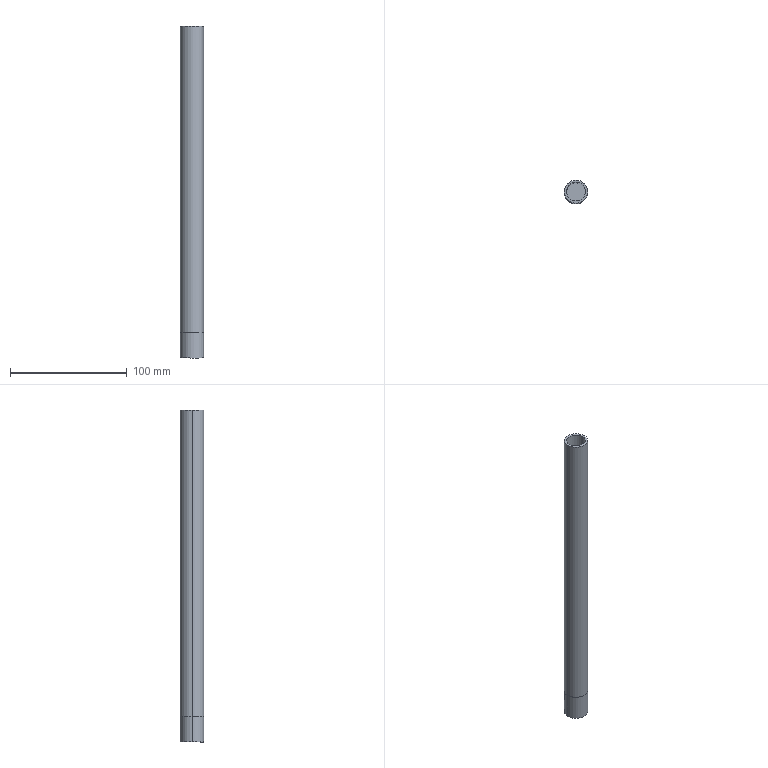Part | SolidWorks | features BaseBody 2 | 2 solids | 17 faces | box 20 x 20 x 284 mm | volume 37985 mm3 | cylinder 10 | plane 5 | cone 2 | commonest cylinder face diameters 16 x4 20 x4 5 x2
STEP:
#1=CARTESIAN_POINT('',(-12.135,0.8028,131.));
#2=VERTEX_POINT('',#1);
#3=CARTESIAN_POINT('',(3.865,0.8028,131.));
#4=VERTEX_POINT('',#3);
#5=CARTESIAN_POINT('',(-4.135,0.8028,131.));
#6=DIRECTION('',(0.,0.,1.));
#7=DIRECTION('',(1.,0.,0.));
#8=AXIS2_PLACEMENT_3D('',#5,#6,#7);
#9=CIRCLE('',#8,8.);
#10=EDGE_CURVE('',#2,#4,#9,.T.);
#11=ORIENTED_EDGE('',*,*,#10,.T.);
#12=CARTESIAN_POINT('',(3.865,0.8028,-131.));
#13=VERTEX_POINT('',#12);
#14=CARTESIAN_POINT('',(3.865,0.8028,131.));
#15=DIRECTION('',(0.,0.,-1.));
#16=VECTOR('',#15,1000.);
#17=LINE('',#14,#16);
#18=EDGE_CURVE('',#4,#13,#17,.T.);
#19=ORIENTED_EDGE('',*,*,#18,.T.);
#20=CARTESIAN_POINT('',(-12.135,0.8028,-131.));
#21=VERTEX_POINT('',#20);
#22=CARTESIAN_POINT('',(-4.135,0.8028,-131.));
#23=DIRECTION('',(0.,0.,1.));
#24=DIRECTION('',(1.,0.,0.));
#25=AXIS2_PLACEMENT_3D('',#22,#23,#24);
#26=CIRCLE('',#25,8.);
#27=EDGE_CURVE('',#21,#13,#26,.T.);
#28=ORIENTED_EDGE('',*,*,#27,.F.);
#29=CARTESIAN_POINT('',(-12.135,0.8028,131.));
#30=DIRECTION('',(0.,0.,-1.));
#31=VECTOR('',#30,1000.);
#32=LINE('',#29,#31);
#33=EDGE_CURVE('',#2,#21,#32,.T.);
#34=ORIENTED_EDGE('',*,*,#33,.F.);
#35=EDGE_LOOP('',(#11,#19,#28,#34));
#36=FACE_OUTER_BOUND('',#35,.T.);
#37=CARTESIAN_POINT('',(-4.135,0.8028,131.));
#38=DIRECTION('',(0.,0.,-1.));
#39=DIRECTION('',(-1.,0.,0.));
#40=AXIS2_PLACEMENT_3D('',#37,#38,#39);
#41=CYLINDRICAL_SURFACE('',#40,8.);
#42=ADVANCED_FACE('',(#36),#41,.F.);
#43=CARTESIAN_POINT('',(5.865,0.8028,131.));
#44=VERTEX_POINT('',#43);
#45=CARTESIAN_POINT('',(-14.135,0.8028,131.));
#46=VERTEX_POINT('',#45);
#47=CARTESIAN_POINT('',(-4.135,0.8028,131.));
#48=DIRECTION('',(0.,0.,1.));
#49=DIRECTION('',(1.,0.,0.));
#50=AXIS2_PLACEMENT_3D('',#47,#48,#49);
#51=CIRCLE('',#50,10.);
#52=EDGE_CURVE('',#44,#46,#51,.T.);
#53=ORIENTED_EDGE('',*,*,#52,.F.);
#54=CARTESIAN_POINT('',(5.865,0.8028,-131.));
#55=VERTEX_POINT('',#54);
#56=CARTESIAN_POINT('',(5.865,0.8028,131.));
#57=DIRECTION('',(0.,0.,-1.));
#58=VECTOR('',#57,1000.);
#59=LINE('',#56,#58);
#60=EDGE_CURVE('',#44,#55,#59,.T.);
#61=ORIENTED_EDGE('',*,*,#60,.T.);
#62=CARTESIAN_POINT('',(-14.135,0.8028,-131.));
#63=VERTEX_POINT('',#62);
#64=CARTESIAN_POINT('',(-4.135,0.8028,-131.));
#65=DIRECTION('',(0.,0.,1.));
#66=DIRECTION('',(1.,0.,0.));
#67=AXIS2_PLACEMENT_3D('',#64,#65,#66);
#68=CIRCLE('',#67,10.);
#69=EDGE_CURVE('',#55,#63,#68,.T.);
#70=ORIENTED_EDGE('',*,*,#69,.T.);
#71=CARTESIAN_POINT('',(-14.135,0.8028,131.));
#72=DIRECTION('',(0.,0.,-1.));
#73=VECTOR('',#72,1000.);
#74=LINE('',#71,#73);
#75=EDGE_CURVE('',#46,#63,#74,.T.);
#76=ORIENTED_EDGE('',*,*,#75,.F.);
#77=EDGE_LOOP('',(#53,#61,#70,#76));
#78=FACE_OUTER_BOUND('',#77,.T.);
#79=CARTESIAN_POINT('',(-4.135,0.8028,131.));
#80=DIRECTION('',(0.,0.,-1.));
#81=DIRECTION('',(-1.,0.,0.));
#82=AXIS2_PLACEMENT_3D('',#79,#80,#81);
#83=CYLINDRICAL_SURFACE('',#82,10.);
#84=ADVANCED_FACE('',(#78),#83,.T.);
#85=CARTESIAN_POINT('',(-4.135,0.8028,131.));
#86=DIRECTION('',(0.,0.,1.));
#87=DIRECTION('',(1.,0.,0.));
#88=AXIS2_PLACEMENT_3D('',#85,#86,#87);
#89=CIRCLE('',#88,10.);
#90=EDGE_CURVE('',#46,#44,#89,.T.);
#91=ORIENTED_EDGE('',*,*,#90,.T.);
#92=ORIENTED_EDGE('',*,*,#52,.T.);
#93=EDGE_LOOP('',(#91,#92));
#94=FACE_OUTER_BOUND('',#93,.T.);
#95=ORIENTED_EDGE('',*,*,#10,.F.);
#96=CARTESIAN_POINT('',(-4.135,0.8028,131.));
#97=DIRECTION('',(0.,0.,1.));
#98=DIRECTION('',(1.,0.,0.));
#99=AXIS2_PLACEMENT_3D('',#96,#97,#98);
#100=CIRCLE('',#99,8.);
#101=EDGE_CURVE('',#4,#2,#100,.T.);
#102=ORIENTED_EDGE('',*,*,#101,.F.);
#103=EDGE_LOOP('',(#95,#102));
#104=FACE_BOUND('',#103,.T.);
#105=CARTESIAN_POINT('',(-4.135,0.8028,131.));
#106=DIRECTION('',(0.,0.,1.));
#107=DIRECTION('',(1.,0.,0.));
#108=AXIS2_PLACEMENT_3D('',#105,#106,#107);
#109=PLANE('',#108);
#110=ADVANCED_FACE('',(#94,#104),#109,.T.);
#111=CARTESIAN_POINT('',(-4.135,0.8028,-131.));
#112=DIRECTION('',(0.,0.,1.));
#113=DIRECTION('',(1.,0.,0.));
#114=AXIS2_PLACEMENT_3D('',#111,#112,#113);
#115=CIRCLE('',#114,10.);
#116=EDGE_CURVE('',#63,#55,#115,.T.);
#117=ORIENTED_EDGE('',*,*,#116,.F.);
#118=ORIENTED_EDGE('',*,*,#69,.F.);
#119=EDGE_LOOP('',(#117,#118));
#120=FACE_OUTER_BOUND('',#119,.T.);
#121=ORIENTED_EDGE('',*,*,#27,.T.);
#122=CARTESIAN_POINT('',(-4.135,0.8028,-131.));
#123=DIRECTION('',(0.,0.,1.));
#124=DIRECTION('',(1.,0.,0.));
#125=AXIS2_PLACEMENT_3D('',#122,#123,#124);
#126=CIRCLE('',#125,8.);
#127=EDGE_CURVE('',#13,#21,#126,.T.);
#128=ORIENTED_EDGE('',*,*,#127,.T.);
#129=EDGE_LOOP('',(#121,#128));
#130=FACE_BOUND('',#129,.T.);
#131=CARTESIAN_POINT('',(-4.135,0.8028,-131.));
#132=DIRECTION('',(0.,0.,1.));
#133=DIRECTION('',(1.,0.,0.));
#134=AXIS2_PLACEMENT_3D('',#131,#132,#133);
#135=PLANE('',#134);
#136=ADVANCED_FACE('',(#120,#130),#135,.F.);
#137=ORIENTED_EDGE('',*,*,#60,.F.);
#138=ORIENTED_EDGE('',*,*,#90,.F.);
#139=ORIENTED_EDGE('',*,*,#75,.T.);
#140=ORIENTED_EDGE('',*,*,#116,.T.);
#141=EDGE_LOOP('',(#137,#138,#139,#140));
#142=FACE_OUTER_BOUND('',#141,.T.);
#143=CARTESIAN_POINT('',(-4.135,0.8028,131.));
#144=DIRECTION('',(0.,0.,-1.));
#145=DIRECTION('',(-1.,0.,0.));
#146=AXIS2_PLACEMENT_3D('',#143,#144,#145);
#147=CYLINDRICAL_SURFACE('',#146,10.);
#148=ADVANCED_FACE('',(#142),#147,.T.);
#149=ORIENTED_EDGE('',*,*,#18,.F.);
#150=ORIENTED_EDGE('',*,*,#101,.T.);
#151=ORIENTED_EDGE('',*,*,#33,.T.);
#152=ORIENTED_EDGE('',*,*,#127,.F.);
#153=EDGE_LOOP('',(#149,#150,#151,#152));
#154=FACE_OUTER_BOUND('',#153,.T.);
#155=CARTESIAN_POINT('',(-4.135,0.8028,131.));
#156=DIRECTION('',(0.,0.,-1.));
#157=DIRECTION('',(-1.,0.,0.));
#158=AXIS2_PLACEMENT_3D('',#155,#156,#157);
#159=CYLINDRICAL_SURFACE('',#158,8.);
#160=ADVANCED_FACE('',(#154),#159,.F.);
#161=CLOSED_SHELL('',(#42,#84,#110,#136,#148,#160));
#162=MANIFOLD_SOLID_BREP('',#161);
#163=CARTESIAN_POINT('',(-1.636,0.8812,-145.));
#164=VERTEX_POINT('',#163);
#165=CARTESIAN_POINT('',(-6.634,0.7244,-145.));
#166=VERTEX_POINT('',#165);
#167=CARTESIAN_POINT('',(-4.135,0.8028,-145.));
#168=DIRECTION('',(0.,0.,-1.));
#169=DIRECTION('',(-0.9995,-0.03135,0.));
#170=AXIS2_PLACEMENT_3D('',#167,#168,#169);
#171=CIRCLE('',#170,2.5);
#172=EDGE_CURVE('',#164,#166,#171,.T.);
#173=ORIENTED_EDGE('',*,*,#172,.F.);
#174=CARTESIAN_POINT('',(-1.636,0.8812,-153.));
#175=VERTEX_POINT('',#174);
#176=CARTESIAN_POINT('',(-1.636,0.8812,-153.));
#177=DIRECTION('',(0.,0.,-1.));
#178=VECTOR('',#177,1000.);
#179=LINE('',#176,#178);
#180=EDGE_CURVE('',#164,#175,#179,.T.);
#181=ORIENTED_EDGE('',*,*,#180,.T.);
#182=CARTESIAN_POINT('',(-6.634,0.7244,-153.));
#183=VERTEX_POINT('',#182);
#184=CARTESIAN_POINT('',(-4.135,0.8028,-153.));
#185=DIRECTION('',(0.,0.,-1.));
#186=DIRECTION('',(-0.9995,-0.03135,0.));
#187=AXIS2_PLACEMENT_3D('',#184,#185,#186);
#188=CIRCLE('',#187,2.5);
#189=EDGE_CURVE('',#175,#183,#188,.T.);
#190=ORIENTED_EDGE('',*,*,#189,.T.);
#191=CARTESIAN_POINT('',(-6.634,0.7244,-153.));
#192=DIRECTION('',(0.,0.,-1.));
#193=VECTOR('',#192,1000.);
#194=LINE('',#191,#193);
#195=EDGE_CURVE('',#166,#183,#194,.T.);
#196=ORIENTED_EDGE('',*,*,#195,.F.);
#197=EDGE_LOOP('',(#173,#181,#190,#196));
#198=FACE_OUTER_BOUND('',#197,.T.);
#199=CARTESIAN_POINT('',(-4.135,0.8028,-153.));
#200=DIRECTION('',(0.,0.,-1.));
#201=DIRECTION('',(-0.9995,-0.03135,0.));
#202=AXIS2_PLACEMENT_3D('',#199,#200,#201);
#203=CYLINDRICAL_SURFACE('',#202,2.5);
#204=ADVANCED_FACE('',(#198),#203,.F.);
#205=CARTESIAN_POINT('',(-4.135,0.8028,-143.498));
#206=VERTEX_POINT('',#205);
#207=CARTESIAN_POINT('',(-6.634,0.7244,-145.));
#208=DIRECTION('',(-0.8567,-0.02688,-0.515));
#209=VECTOR('',#208,1000.);
#210=LINE('',#207,#209);
#211=EDGE_CURVE('',#206,#166,#210,.T.);
#212=ORIENTED_EDGE('',*,*,#211,.F.);
#213=CARTESIAN_POINT('',(-1.636,0.8812,-145.));
#214=DIRECTION('',(0.8567,0.02688,-0.515));
#215=VECTOR('',#214,1000.);
#216=LINE('',#213,#215);
#217=EDGE_CURVE('',#206,#164,#216,.T.);
#218=ORIENTED_EDGE('',*,*,#217,.T.);
#219=ORIENTED_EDGE('',*,*,#172,.T.);
#220=EDGE_LOOP('',(#212,#218,#219));
#221=FACE_OUTER_BOUND('',#220,.T.);
#222=CARTESIAN_POINT('',(-4.135,0.8028,-145.));
#223=DIRECTION('',(0.,0.,-1.));
#224=DIRECTION('',(-0.9995,-0.03135,0.));
#225=AXIS2_PLACEMENT_3D('',#222,#223,#224);
#226=CONICAL_SURFACE('',#225,2.5,1.03);
#227=ADVANCED_FACE('',(#221),#226,.F.);
#228=CARTESIAN_POINT('',(5.86,1.116,-153.));
#229=VERTEX_POINT('',#228);
#230=CARTESIAN_POINT('',(-14.13,0.4893,-153.));
#231=VERTEX_POINT('',#230);
#232=CARTESIAN_POINT('',(-4.135,0.8028,-153.));
#233=DIRECTION('',(0.,0.,1.));
#234=DIRECTION('',(0.9995,0.03135,0.));
#235=AXIS2_PLACEMENT_3D('',#232,#233,#234);
#236=CIRCLE('',#235,10.);
#237=EDGE_CURVE('',#229,#231,#236,.T.);
#238=ORIENTED_EDGE('',*,*,#237,.T.);
#239=CARTESIAN_POINT('',(-14.13,0.4893,-131.));
#240=VERTEX_POINT('',#239);
#241=CARTESIAN_POINT('',(-14.13,0.4893,-153.));
#242=DIRECTION('',(0.,0.,1.));
#243=VECTOR('',#242,1000.);
#244=LINE('',#241,#243);
#245=EDGE_CURVE('',#231,#240,#244,.T.);
#246=ORIENTED_EDGE('',*,*,#245,.T.);
#247=CARTESIAN_POINT('',(5.86,1.116,-131.));
#248=VERTEX_POINT('',#247);
#249=CARTESIAN_POINT('',(-4.135,0.8028,-131.));
#250=DIRECTION('',(0.,0.,1.));
#251=DIRECTION('',(0.9995,0.03135,0.));
#252=AXIS2_PLACEMENT_3D('',#249,#250,#251);
#253=CIRCLE('',#252,10.);
#254=EDGE_CURVE('',#248,#240,#253,.T.);
#255=ORIENTED_EDGE('',*,*,#254,.F.);
#256=CARTESIAN_POINT('',(5.86,1.116,-153.));
#257=DIRECTION('',(0.,0.,1.));
#258=VECTOR('',#257,1000.);
#259=LINE('',#256,#258);
#260=EDGE_CURVE('',#229,#248,#259,.T.);
#261=ORIENTED_EDGE('',*,*,#260,.F.);
#262=EDGE_LOOP('',(#238,#246,#255,#261));
#263=FACE_OUTER_BOUND('',#262,.T.);
#264=CARTESIAN_POINT('',(-4.135,0.8028,-153.));
#265=DIRECTION('',(0.,0.,1.));
#266=DIRECTION('',(0.9995,0.03135,0.));
#267=AXIS2_PLACEMENT_3D('',#264,#265,#266);
#268=CYLINDRICAL_SURFACE('',#267,10.);
#269=ADVANCED_FACE('',(#263),#268,.T.);
#270=CARTESIAN_POINT('',(3.861,1.054,-123.));
#271=VERTEX_POINT('',#270);
#272=CARTESIAN_POINT('',(-12.131,0.552,-123.));
#273=VERTEX_POINT('',#272);
#274=CARTESIAN_POINT('',(-4.135,0.8028,-123.));
#275=DIRECTION('',(0.,0.,1.));
#276=DIRECTION('',(0.9995,0.03135,0.));
#277=AXIS2_PLACEMENT_3D('',#274,#275,#276);
#278=CIRCLE('',#277,8.);
#279=EDGE_CURVE('',#271,#273,#278,.T.);
#280=ORIENTED_EDGE('',*,*,#279,.F.);
#281=CARTESIAN_POINT('',(3.861,1.054,-131.));
#282=VERTEX_POINT('',#281);
#283=CARTESIAN_POINT('',(3.861,1.054,-123.));
#284=DIRECTION('',(0.,0.,-1.));
#285=VECTOR('',#284,1000.);
#286=LINE('',#283,#285);
#287=EDGE_CURVE('',#271,#282,#286,.T.);
#288=ORIENTED_EDGE('',*,*,#287,.T.);
#289=CARTESIAN_POINT('',(-12.131,0.552,-131.));
#290=VERTEX_POINT('',#289);
#291=CARTESIAN_POINT('',(-4.135,0.8028,-131.));
#292=DIRECTION('',(0.,0.,1.));
#293=DIRECTION('',(0.9995,0.03135,0.));
#294=AXIS2_PLACEMENT_3D('',#291,#292,#293);
#295=CIRCLE('',#294,8.);
#296=EDGE_CURVE('',#282,#290,#295,.T.);
#297=ORIENTED_EDGE('',*,*,#296,.T.);
#298=CARTESIAN_POINT('',(-12.131,0.552,-123.));
#299=DIRECTION('',(0.,0.,-1.));
#300=VECTOR('',#299,1000.);
#301=LINE('',#298,#300);
#302=EDGE_CURVE('',#273,#290,#301,.T.);
#303=ORIENTED_EDGE('',*,*,#302,.F.);
#304=EDGE_LOOP('',(#280,#288,#297,#303));
#305=FACE_OUTER_BOUND('',#304,.T.);
#306=CARTESIAN_POINT('',(-4.135,0.8028,-123.));
#307=DIRECTION('',(0.,0.,-1.));
#308=DIRECTION('',(-0.9995,-0.03135,0.));
#309=AXIS2_PLACEMENT_3D('',#306,#307,#308);
#310=CYLINDRICAL_SURFACE('',#309,8.);
#311=ADVANCED_FACE('',(#305),#310,.T.);
#312=ORIENTED_EDGE('',*,*,#287,.F.);
#313=CARTESIAN_POINT('',(-4.135,0.8028,-123.));
#314=DIRECTION('',(0.,0.,1.));
#315=DIRECTION('',(0.9995,0.03135,0.));
#316=AXIS2_PLACEMENT_3D('',#313,#314,#315);
#317=CIRCLE('',#316,8.);
#318=EDGE_CURVE('',#273,#271,#317,.T.);
#319=ORIENTED_EDGE('',*,*,#318,.F.);
#320=ORIENTED_EDGE('',*,*,#302,.T.);
#321=CARTESIAN_POINT('',(-4.135,0.8028,-131.));
#322=DIRECTION('',(0.,0.,1.));
#323=DIRECTION('',(0.9995,0.03135,0.));
#324=AXIS2_PLACEMENT_3D('',#321,#322,#323);
#325=CIRCLE('',#324,8.);
#326=EDGE_CURVE('',#290,#282,#325,.T.);
#327=ORIENTED_EDGE('',*,*,#326,.T.);
#328=EDGE_LOOP('',(#312,#319,#320,#327));
#329=FACE_OUTER_BOUND('',#328,.T.);
#330=CARTESIAN_POINT('',(-4.135,0.8028,-123.));
#331=DIRECTION('',(0.,0.,-1.));
#332=DIRECTION('',(-0.9995,-0.03135,0.));
#333=AXIS2_PLACEMENT_3D('',#330,#331,#332);
#334=CYLINDRICAL_SURFACE('',#333,8.);
#335=ADVANCED_FACE('',(#329),#334,.T.);
#336=ORIENTED_EDGE('',*,*,#318,.T.);
#337=ORIENTED_EDGE('',*,*,#279,.T.);
#338=EDGE_LOOP('',(#336,#337));
#339=FACE_OUTER_BOUND('',#338,.T.);
#340=CARTESIAN_POINT('',(-4.135,0.8028,-123.));
#341=DIRECTION('',(0.,0.,1.));
#342=DIRECTION('',(0.9995,0.03135,0.));
#343=AXIS2_PLACEMENT_3D('',#340,#341,#342);
#344=PLANE('',#343);
#345=ADVANCED_FACE('',(#339),#344,.T.);
#346=ORIENTED_EDGE('',*,*,#245,.F.);
#347=CARTESIAN_POINT('',(-4.135,0.8028,-153.));
#348=DIRECTION('',(0.,0.,1.));
#349=DIRECTION('',(0.9995,0.03135,0.));
#350=AXIS2_PLACEMENT_3D('',#347,#348,#349);
#351=CIRCLE('',#350,10.);
#352=EDGE_CURVE('',#231,#229,#351,.T.);
#353=ORIENTED_EDGE('',*,*,#352,.T.);
#354=ORIENTED_EDGE('',*,*,#260,.T.);
#355=CARTESIAN_POINT('',(-4.135,0.8028,-131.));
#356=DIRECTION('',(0.,0.,1.));
#357=DIRECTION('',(0.9995,0.03135,0.));
#358=AXIS2_PLACEMENT_3D('',#355,#356,#357);
#359=CIRCLE('',#358,10.);
#360=EDGE_CURVE('',#240,#248,#359,.T.);
#361=ORIENTED_EDGE('',*,*,#360,.F.);
#362=EDGE_LOOP('',(#346,#353,#354,#361));
#363=FACE_OUTER_BOUND('',#362,.T.);
#364=CARTESIAN_POINT('',(-4.135,0.8028,-153.));
#365=DIRECTION('',(0.,0.,1.));
#366=DIRECTION('',(0.9995,0.03135,0.));
#367=AXIS2_PLACEMENT_3D('',#364,#365,#366);
#368=CYLINDRICAL_SURFACE('',#367,10.);
#369=ADVANCED_FACE('',(#363),#368,.T.);
#370=CARTESIAN_POINT('',(-4.135,0.8028,-153.));
#371=DIRECTION('',(0.,0.,-1.));
#372=DIRECTION('',(-0.9995,-0.03135,0.));
#373=AXIS2_PLACEMENT_3D('',#370,#371,#372);
#374=CIRCLE('',#373,2.5);
#375=EDGE_CURVE('',#183,#175,#374,.T.);
#376=ORIENTED_EDGE('',*,*,#375,.F.);
#377=ORIENTED_EDGE('',*,*,#189,.F.);
#378=EDGE_LOOP('',(#376,#377));
#379=FACE_BOUND('',#378,.T.);
#380=ORIENTED_EDGE('',*,*,#237,.F.);
#381=ORIENTED_EDGE('',*,*,#352,.F.);
#382=EDGE_LOOP('',(#380,#381));
#383=FACE_OUTER_BOUND('',#382,.T.);
#384=CARTESIAN_POINT('',(-4.135,0.8028,-153.));
#385=DIRECTION('',(0.,0.,1.));
#386=DIRECTION('',(0.9995,0.03135,0.));
#387=AXIS2_PLACEMENT_3D('',#384,#385,#386);
#388=PLANE('',#387);
#389=ADVANCED_FACE('',(#379,#383),#388,.F.);
#390=ORIENTED_EDGE('',*,*,#326,.F.);
#391=ORIENTED_EDGE('',*,*,#296,.F.);
#392=EDGE_LOOP('',(#390,#391));
#393=FACE_BOUND('',#392,.T.);
#394=ORIENTED_EDGE('',*,*,#254,.T.);
#395=ORIENTED_EDGE('',*,*,#360,.T.);
#396=EDGE_LOOP('',(#394,#395));
#397=FACE_OUTER_BOUND('',#396,.T.);
#398=CARTESIAN_POINT('',(-4.135,0.8028,-131.));
#399=DIRECTION('',(0.,0.,1.));
#400=DIRECTION('',(0.9995,0.03135,0.));
#401=AXIS2_PLACEMENT_3D('',#398,#399,#400);
#402=PLANE('',#401);
#403=ADVANCED_FACE('',(#393,#397),#402,.T.);
#404=ORIENTED_EDGE('',*,*,#217,.F.);
#405=ORIENTED_EDGE('',*,*,#211,.T.);
#406=CARTESIAN_POINT('',(-4.135,0.8028,-145.));
#407=DIRECTION('',(0.,0.,-1.));
#408=DIRECTION('',(-0.9995,-0.03135,0.));
#409=AXIS2_PLACEMENT_3D('',#406,#407,#408);
#410=CIRCLE('',#409,2.5);
#411=EDGE_CURVE('',#166,#164,#410,.T.);
#412=ORIENTED_EDGE('',*,*,#411,.T.);
#413=EDGE_LOOP('',(#404,#405,#412));
#414=FACE_OUTER_BOUND('',#413,.T.);
#415=CARTESIAN_POINT('',(-4.135,0.8028,-145.));
#416=DIRECTION('',(0.,0.,-1.));
#417=DIRECTION('',(-0.9995,-0.03135,0.));
#418=AXIS2_PLACEMENT_3D('',#415,#416,#417);
#419=CONICAL_SURFACE('',#418,2.5,1.03);
#420=ADVANCED_FACE('',(#414),#419,.F.);
#421=ORIENTED_EDGE('',*,*,#180,.F.);
#422=ORIENTED_EDGE('',*,*,#411,.F.);
#423=ORIENTED_EDGE('',*,*,#195,.T.);
#424=ORIENTED_EDGE('',*,*,#375,.T.);
#425=EDGE_LOOP('',(#421,#422,#423,#424));
#426=FACE_OUTER_BOUND('',#425,.T.);
#427=CARTESIAN_POINT('',(-4.135,0.8028,-153.));
#428=DIRECTION('',(0.,0.,-1.));
#429=DIRECTION('',(-0.9995,-0.03135,0.));
#430=AXIS2_PLACEMENT_3D('',#427,#428,#429);
#431=CYLINDRICAL_SURFACE('',#430,2.5);
#432=ADVANCED_FACE('',(#426),#431,.F.);
#433=CLOSED_SHELL('',(#204,#227,#269,#311,#335,#345,#369,#389,#403,#420,#432));
#434=MANIFOLD_SOLID_BREP('',#433);
#435=CARTESIAN_POINT('',(0.,0.,0.));
#436=DIRECTION('',(0.,0.,1.));
#437=DIRECTION('',(1.,0.,0.));
#438=AXIS2_PLACEMENT_3D('',#435,#436,#437);
#439=(LENGTH_UNIT()NAMED_UNIT(*)SI_UNIT(.MILLI.,.METRE.));
#440=UNCERTAINTY_MEASURE_WITH_UNIT(LENGTH_MEASURE(0.00001),#439,'','');
#441=(NAMED_UNIT(*)PLANE_ANGLE_UNIT()SI_UNIT($,.RADIAN.));
#442=(NAMED_UNIT(*)SI_UNIT($,.STERADIAN.)SOLID_ANGLE_UNIT());
#443=(GEOMETRIC_REPRESENTATION_CONTEXT(3)GLOBAL_UNCERTAINTY_ASSIGNED_CONTEXT((#440))GLOBAL_UNIT_ASSIGNED_CONTEXT((#439,#441,#442))REPRESENTATION_CONTEXT('',''));
#444=ADVANCED_BREP_SHAPE_REPRESENTATION('',(#162,#434,#438),#443);